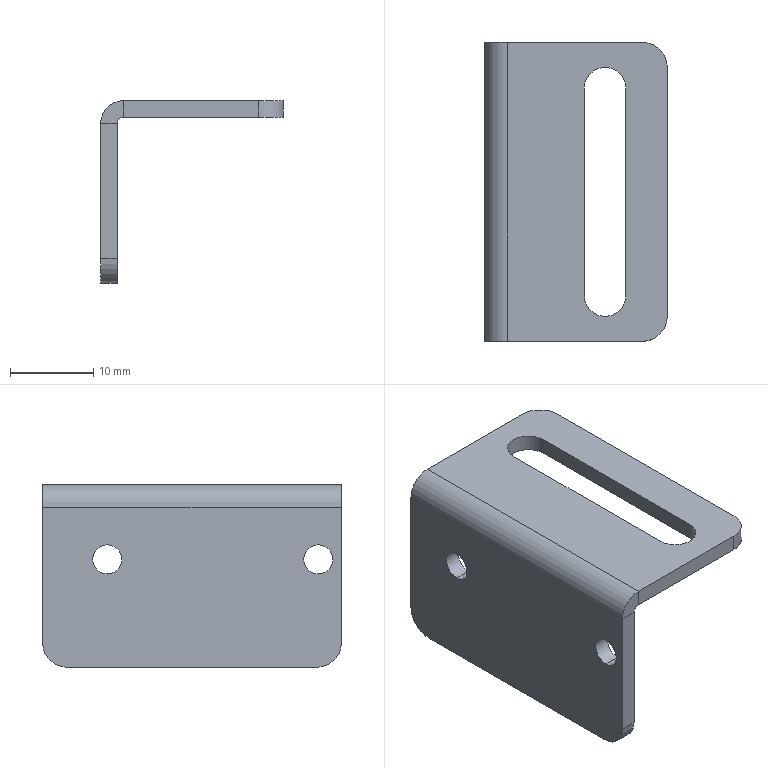Part | STEP file | ND25021-01-JDKM-11-BJ | 1 solid | 26 faces | box 22 x 36 x 22 mm | volume 2627 mm3 | plane 14 | cylinder 12 | commonest cylinder face diameters 3.5 x4 6 x4 5 x2 1.473 x1 5.473 x1